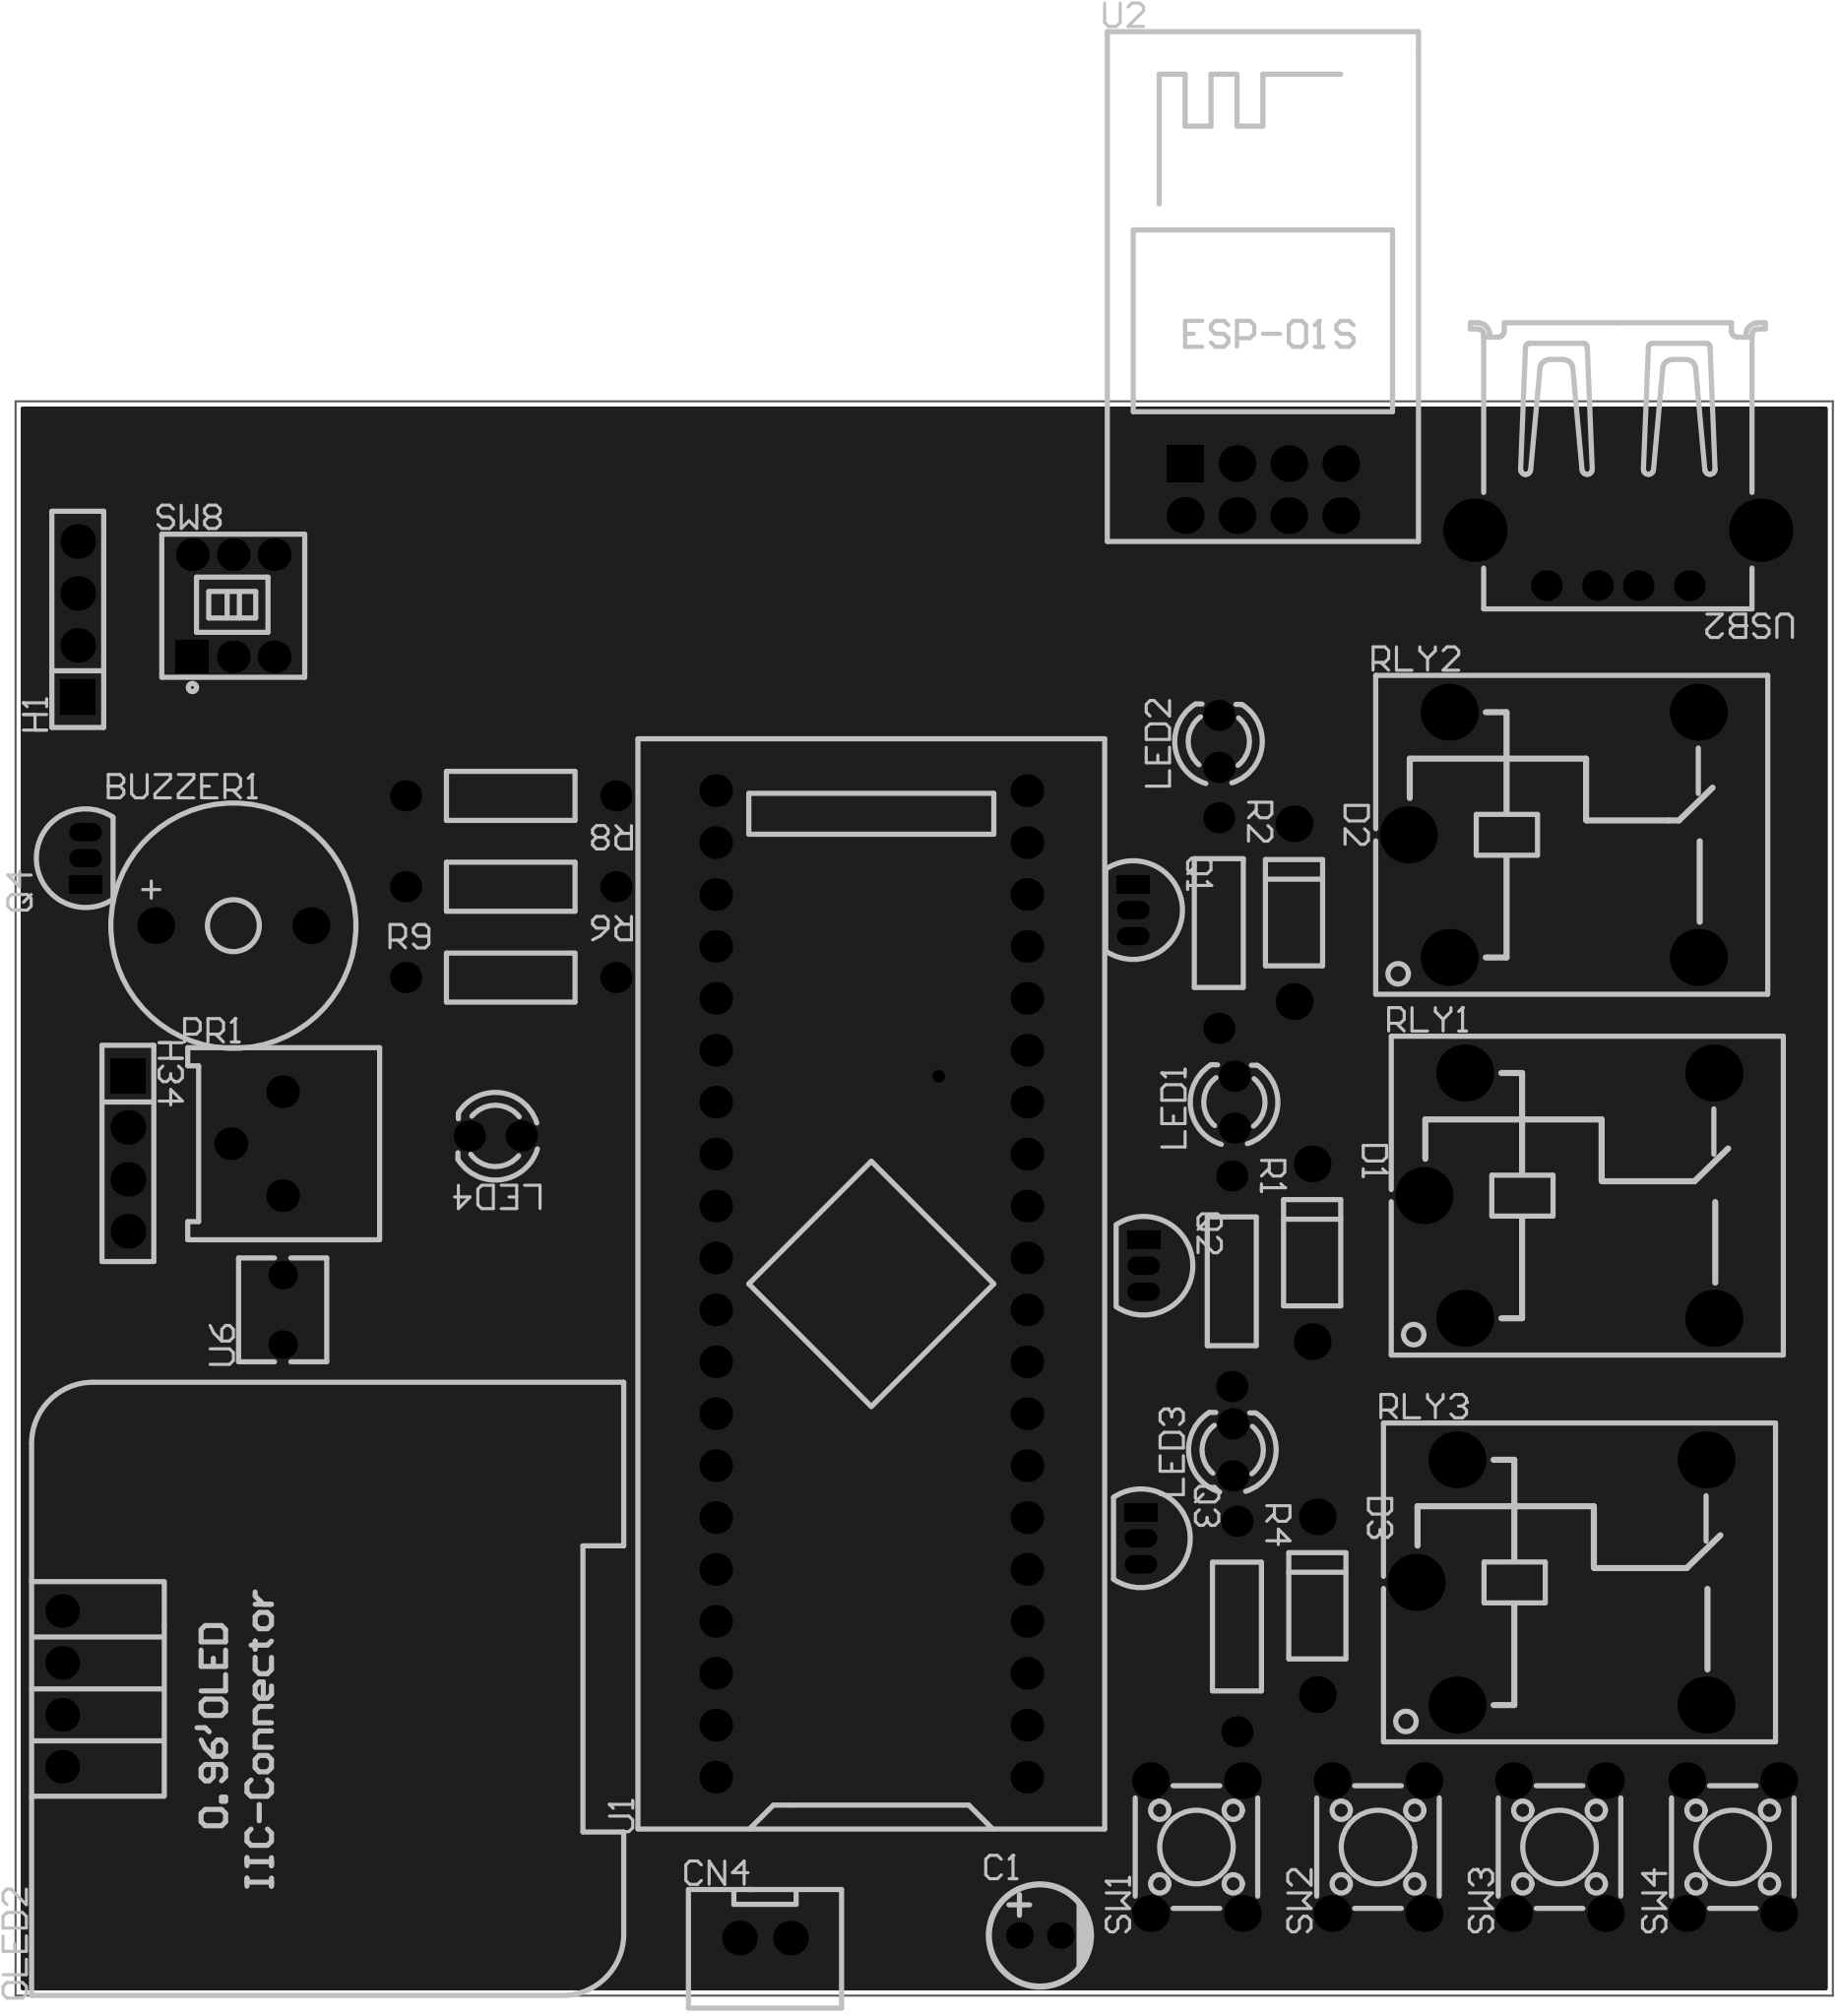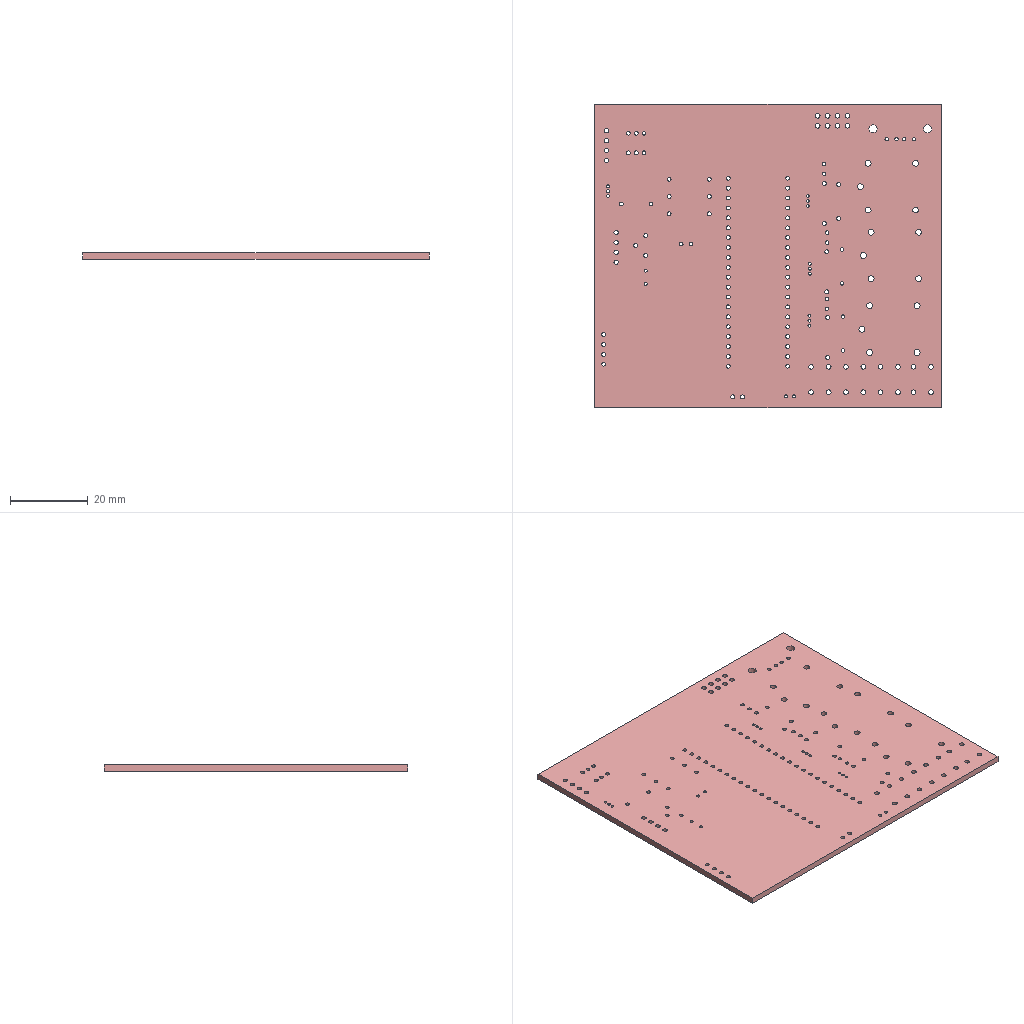Circuit board layout | Altium Designer | box 89 x 78 x 1.6 mm
Layer stack:
# Altium Designer layer stack of  (unit mm; dielectric type: 0 none, 1 core, 2 prepreg, 3 surface material)
index,name,kind,layer,copper_thickness_mm,dielectric_type,dielectric_thickness_mm,dielectric_material,dielectric_constant
0,Top Paste Mask Layer,other,,,,,,
1,Top Silkscreen Layer,other,,,,,,
2,Top Solder Mask Layer,dielectric,,,3,0.01,,3.3
3,Top Layer,copper,Top Layer,0.035,,,,
4,Dielectric1,dielectric,,,3,1.51,FR4,4.5
5,Bottom Layer,copper,Bottom Layer,0.035,,,,
6,Bottom Solder Mask Layer,dielectric,,,3,0.01,,3.3
7,Bottom Silkscreen Layer,other,,,,,,
8,Bottom Paste Mask Layer,other,,,,,,
# drill layer pairs: low layer,high layer
drill_pair,Top Layer,Bottom Layer
Part placement:
Designator,Comment,Layer,Footprint,Center-X(mm),Center-Y(mm),Rotation
BUZZER1,2.3kHz,TopLayer,BUZ-TH_BD12.0-P7.60-D0.6-FD,118.364,183.642,0
C1,10uF,TopLayer,CAP-TH_BD5.0-P2.00-D0.8-FD-10UF50VC110GL,157.861,134.239,0
CN4,XH2.54*2P_Through-hole,TopLayer,CONN-TH_2P-P2.50-XH2.54-2P,144.399,134.112,0
H34,,TopLayer,HDR-TH_4P-P2.54-V-F,113.198,172.5,270
LED1,,TopLayer,LED_TH-3mm,167.386,175.006,90
LED2,,TopLayer,LED_TH-3mm,166.624,192.659,90
LED3,,TopLayer,LED_TH-3mm,167.303,157.998,90
LED4,,TopLayer,LED_TH-3mm,131.191,173.355,180
OLED2,,TopLayer,0.96OLED_4P,109.982,146.304,90
Q1,,TopLayer,S8050_TO_92,162.433,184.404,270
Q2,,TopLayer,S8050_TO_92,162.941,167.005,270
Q3,,TopLayer,S8050_TO_92,162.814,153.67,270
Q4,,TopLayer,S8050_TO_92,111.125,186.944,90
R1,1kΩ,TopLayer,Res_1/4W,167.259,166.243,270
R2,1kΩ,TopLayer,Res_1/4W,166.624,183.769,270
R4,1kΩ,TopLayer,Res_1/4W,167.513,149.352,270
R6,1kΩ,TopLayer,Res_1/4W,131.947,185.547,180
R8,1kΩ,TopLayer,Res_1/4W,131.947,189.992,180
R9,120,TopLayer,Res_1/4W,131.947,181.102,0
RLY1,SRD-05VDC-SL-C,TopLayer,RELAY-TH_SRD-XXVDC-XL-C,183.769,170.434,0
RLY2,SRD-05VDC-SL-C,TopLayer,RELAY-TH_SRD-XXVDC-XL-C,183.007,188.087,0
RLY3,SRD-05VDC-SL-C,TopLayer,RELAY-TH_SRD-XXVDC-XL-C,183.388,151.511,0
SW1,,TopLayer,SW-TH_4P-L6.0-W6.0-P4.50-LS6.5,165.53,138.565,90
SW2,,TopLayer,SW-TH_4P-L6.0-W6.0-P4.50-LS6.5,174.42,138.565,90
SW3,,TopLayer,SW-TH_4P-L6.0-W6.0-P4.50-LS6.5,183.31,138.565,90
SW4,,TopLayer,SW-TH_4P-L6.0-W6.0-P4.50-LS6.5,191.794,138.565,90
SW8,TK-6700-1,TopLayer,SW-TH_TK-6700-1,118.358,199.294,0
U1,STM32F103C8T6-Card,TopLayer,CONN-TH_L53.3-W22.9_STM32F103C8T6-CARD,149.606,166.116,90
U2,ESP-01S,TopLayer,WIFIM-TH_ESP-01S,168.783,204.978,0
U6,光敏电阻-5MM,TopLayer,RES-TH_L4.9-W4.3-P3.4,120.777,164.846,90
USB2,,TopLayer,USB__Type-A,186.166,201.634,180
D1,,TopLayer,DO_1N4007,171.196,167.64,270
D2,,TopLayer,DO_1N4007,170.307,184.277,270
D3,,TopLayer,DO_1N4007,171.45,150.368,270
PR1,10K,TopLayer,R_3386P,119.507,172.974,0
H1,,TopLayer,HDR-TH_4P-P2.54-V-F,110.744,198.628,90
Pad and via stacks:
# Altium Designer via and pad stacks of  (unit mm). Each distinct definition once, with the count of objects using it.
# via: kind,start_layer,end_layer,hole_mm,diameter_mm,mode(0 simple;1 top-mid-bottom;2 full stack),diameter_per_layer,count,example_net
# pad: kind,layer,hole_mm,hole_type(0 round;1 square;2 slot),plating,top_size,top_shape(1 round;2 rect;3 octagon;9 rounded rect),mid_size,bottom_size,mode,footprint,size_per_layer,count,example
pad,Multi-Layer,1,0,plated,1.8x1.8,1,1.8x1.8,1.8x1.8,0,BUZ-TH_BD12.0-P7.60-D0.6-FD,,2,BUZZER1.2
pad,Multi-Layer,0.8,0,plated,1.3x1.3,1,1.3x1.3,1.3x1.3,0,CAP-TH_BD5.0-P2.00-D0.8-FD-10UF50VC110GL,,2,C1.2
pad,Multi-Layer,1.05,0,plated,1.7x1.7,1,1.7x1.7,1.7x1.7,0,CONN-TH_2P-P2.50-XH2.54-2P,,2,CN4.2
pad,Multi-Layer,1.1,0,plated,1.7x1.7,2,1.7x1.7,1.7x1.7,0,HDR-TH_4P-P2.54-V-F,,2,H34.1
pad,Multi-Layer,1.1,0,plated,1.7x1.7,1,1.7x1.7,1.7x1.7,0,HDR-TH_4P-P2.54-V-F,,6,H34.2
pad,Multi-Layer,0.9144,0,plated,1.524x1.524,1,1.524x1.524,1.524x1.524,0,LED_TH-3mm,,8,LED1.1
pad,Multi-Layer,1,0,plated,1.65x1.65,1,1.65x1.65,1.65x1.65,0,0.96OLED_4P,,4,OLED2.4
pad,Multi-Layer,0.701,0,plated,0.8992x1.6,2,0.8992x1.6,0.8992x1.6,0,S8050_TO_92,,4,Q1.1
pad,Multi-Layer,0.701,0,plated,0.8992x1.6,1,0.8992x1.6,0.8992x1.6,0,S8050_TO_92,,8,Q1.2
pad,Multi-Layer,1,0,plated,1.524x1.524,1,1.524x1.524,1.524x1.524,0,Res_1/4W,,12,R1.1
pad,Multi-Layer,1.524,0,plated,2.794x2.794,1,2.794x2.794,2.794x2.794,0,RELAY-TH_SRD-XXVDC-XL-C,,15,RLY1.2
pad,Multi-Layer,1.2,0,plated,1.8x1.8,1,1.8x1.8,1.8x1.8,0,SW-TH_4P-L6.0-W6.0-P4.50-LS6.5,,16,SW1.1
pad,Multi-Layer,1,0,plated,1.6x1.6,2,1.6x1.6,1.6x1.6,0,SW-TH_TK-6700-1,,1,SW8.1
pad,Multi-Layer,1,0,plated,1.6x1.6,1,1.6x1.6,1.6x1.6,0,SW-TH_TK-6700-1,,5,SW8.2
pad,Multi-Layer,1,0,plated,1.6x1.6,1,1.6x1.6,1.6x1.6,0,CONN-TH_L53.3-W22.9_STM32F103C8T6-CARD,,40,U1.1
pad,Multi-Layer,1.2,0,plated,1.8x1.8,2,1.8x1.8,1.8x1.8,0,WIFIM-TH_ESP-01S,,1,U2.1
pad,Multi-Layer,1.2,0,plated,1.8x1.8,1,1.8x1.8,1.8x1.8,0,WIFIM-TH_ESP-01S,,7,U2.2
pad,Multi-Layer,0.8,0,plated,1.4x1.4,1,1.4x1.4,1.4x1.4,0,RES-TH_L4.9-W4.3-P3.4,,2,U6.1
pad,Multi-Layer,2.1,0,plated,3.1x3.1,1,3.1x3.1,3.1x3.1,0,USB_ Type-A,,2,USB2.SH2
pad,Multi-Layer,0.9,0,plated,1.5x1.5,1,1.5x1.5,1.5x1.5,0,USB_ Type-A,,4,USB2.1
pad,Multi-Layer,1,0,plated,1.8x1.8,1,1.8x1.8,1.8x1.8,0,DO_1N4007,,6,D1.1
pad,Multi-Layer,1.001,0,plated,1.6x1.6,1,1.6x1.6,1.6x1.6,0,R_3386P,,3,PR1.2
via,Top Layer,Bottom Layer,0.3048,0.61,0,,1,PB8
Copper pours:
name,layer,net,type(0 solid;1 hatched;2 none)
Top Layer-GND,Top Layer,GND,0
Bottom Layer-GND,Bottom Layer,GND,0
Design rules, without the lines most boards share:
# Altium Designer design rules of  (exported by Altium Designer, unit mm)
# columns: name | kind | enabled | priority | scope1 | scope2 | descriptor | typed fields (field=value)
Copper_copperRegion_copperThickness1oz | 0 | disabled | 4 | All | All | Clearance Constraint (Gap=5.984mil) (Disabled)(All),(All) | gap=0.152
Copper_copperRegion_copperThickness1oz_1 | 63 | disabled | 4 | All | All | Board Clearance Constraint (Gap=0mil) (Disabled)(All) |
Copper_copperRegion_Copper_copperRegion | 0 | disabled | 5 | All | All | Clearance Constraint (Gap=5.984mil) (Disabled)(All),(All) | gap=0.152
Copper_copperRegion_Copper_copperRegion_1 | 63 | disabled | 5 | All | All | Board Clearance Constraint (Gap=0mil) (Disabled)(All) |
copperThickness1oz | 0 | enabled | 6 | All | All | Clearance Constraint (Gap=5.984mil) (All),(All) | gap=0.152
copperThickness1oz_1 | 63 | enabled | 6 | All | All | Board Clearance Constraint (Gap=0mil) (All) |
copperRegion_copperThickness1oz | 20 | disabled | 1 | All | All | Polygon Connect Rule(Relief Connect )(Conductor Width=10mil) (Relief Angle=90 Angle) (Entries=4) (Air Gap Width=10mil) (Disabled)(All),(All) | connect_style(0=relief,1=direct,2=none)=0 relief_conductor_width=0.254 relief_entries=4
copperRegion_Copper_copperRegion | 20 | disabled | 2 | All | All | Polygon Connect Rule(Relief Connect )(Conductor Width=10mil) (Relief Angle=90 Angle) (Entries=4) (Air Gap Width=10mil) (Disabled)(All),(All) | connect_style(0=relief,1=direct,2=none)=0 relief_conductor_width=0.254 relief_entries=4
copperRegion | 20 | enabled | 3 | (InNet('GND')) | All | Polygon Connect Rule(Relief Connect )(Conductor Width=10mil) (Relief Angle=90 Angle) (Entries=4) (Air Gap Width=10mil) ((InNet('GND'))),(All) | connect_style(0=relief,1=direct,2=none)=0 relief_conductor_width=0.254 relief_entries=4